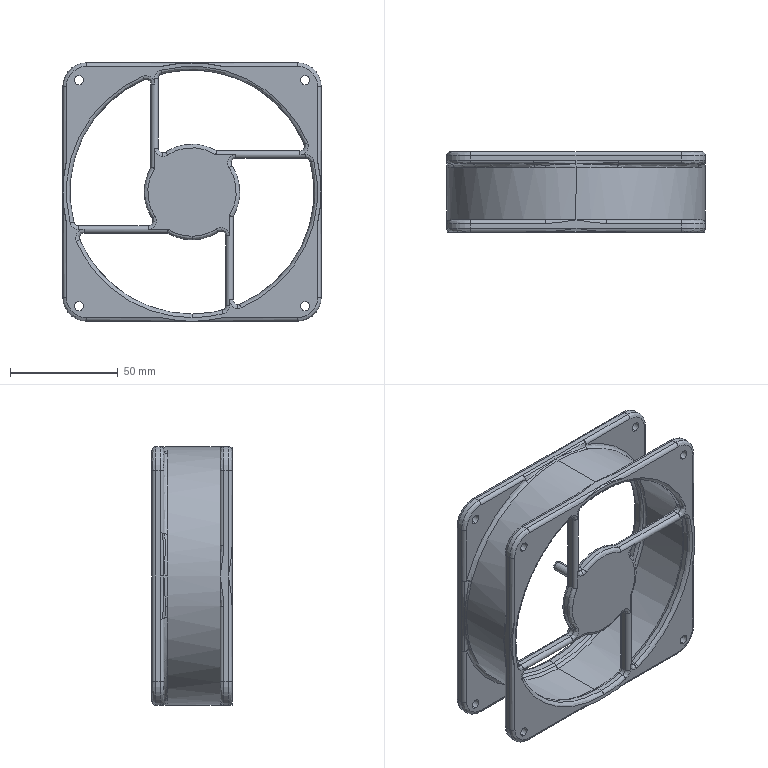Part | SolidWorks | features BaseBody 1, ICE 1, Scale 1 | 1 solid | 241 faces | box 120.002 x 37.222 x 120.002 mm | volume 72632 mm3 | spline 108 | cylinder 97 | plane 36 | commonest cylinder face diameters 3.333 x36 4.3 x16 4.444 x16 22.222 x8 113.333 x7 120 x7